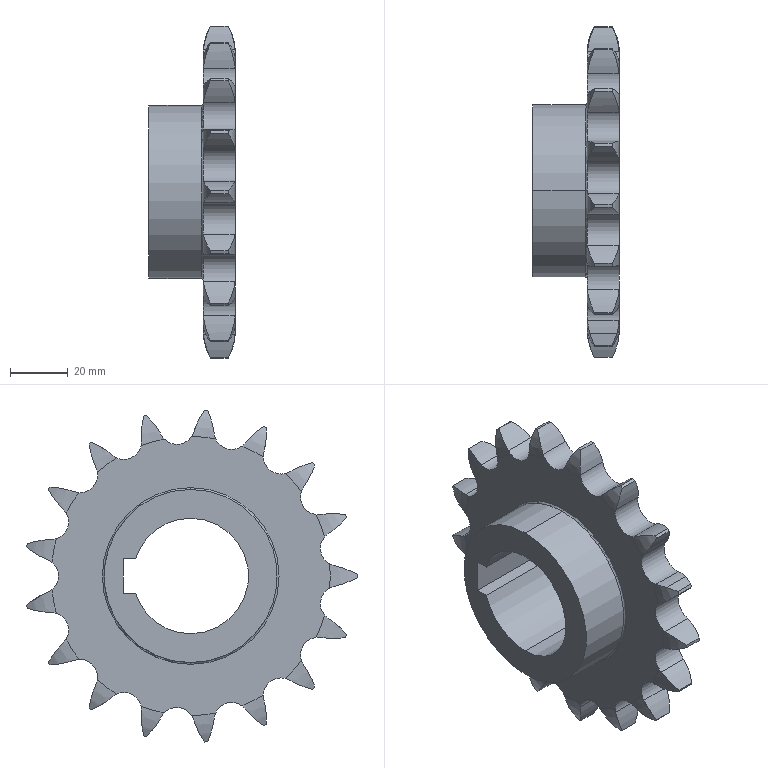Part | SolidWorks | features ICE 4, BaseBody 1, Fillet 1, RevCut 1 | 1 solid | 122 faces | box 30.001 x 114.527 x 115.015 mm | volume 100872 mm3 | cylinder 80 | spline 34 | plane 6 | torus 2 | commonest cylinder face diameters 55.039 x35 12.191 x23 115.416 x17 40 x3 60 x2